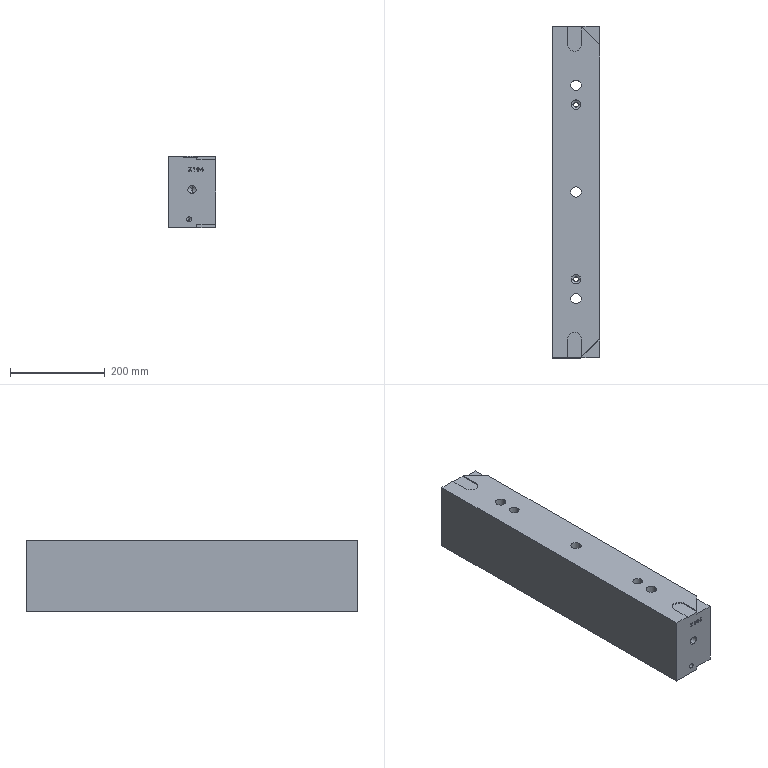Part | Creo | 1 solid | 217 faces | box 100 x 700 x 150 mm | volume 10187083 mm3 | plane 139 | cylinder 31 | other 29 | cone 18 | commonest cylinder face diameters 20 x8 22 x6 10 x4 14 x4 17.5 x4 10.2 x2